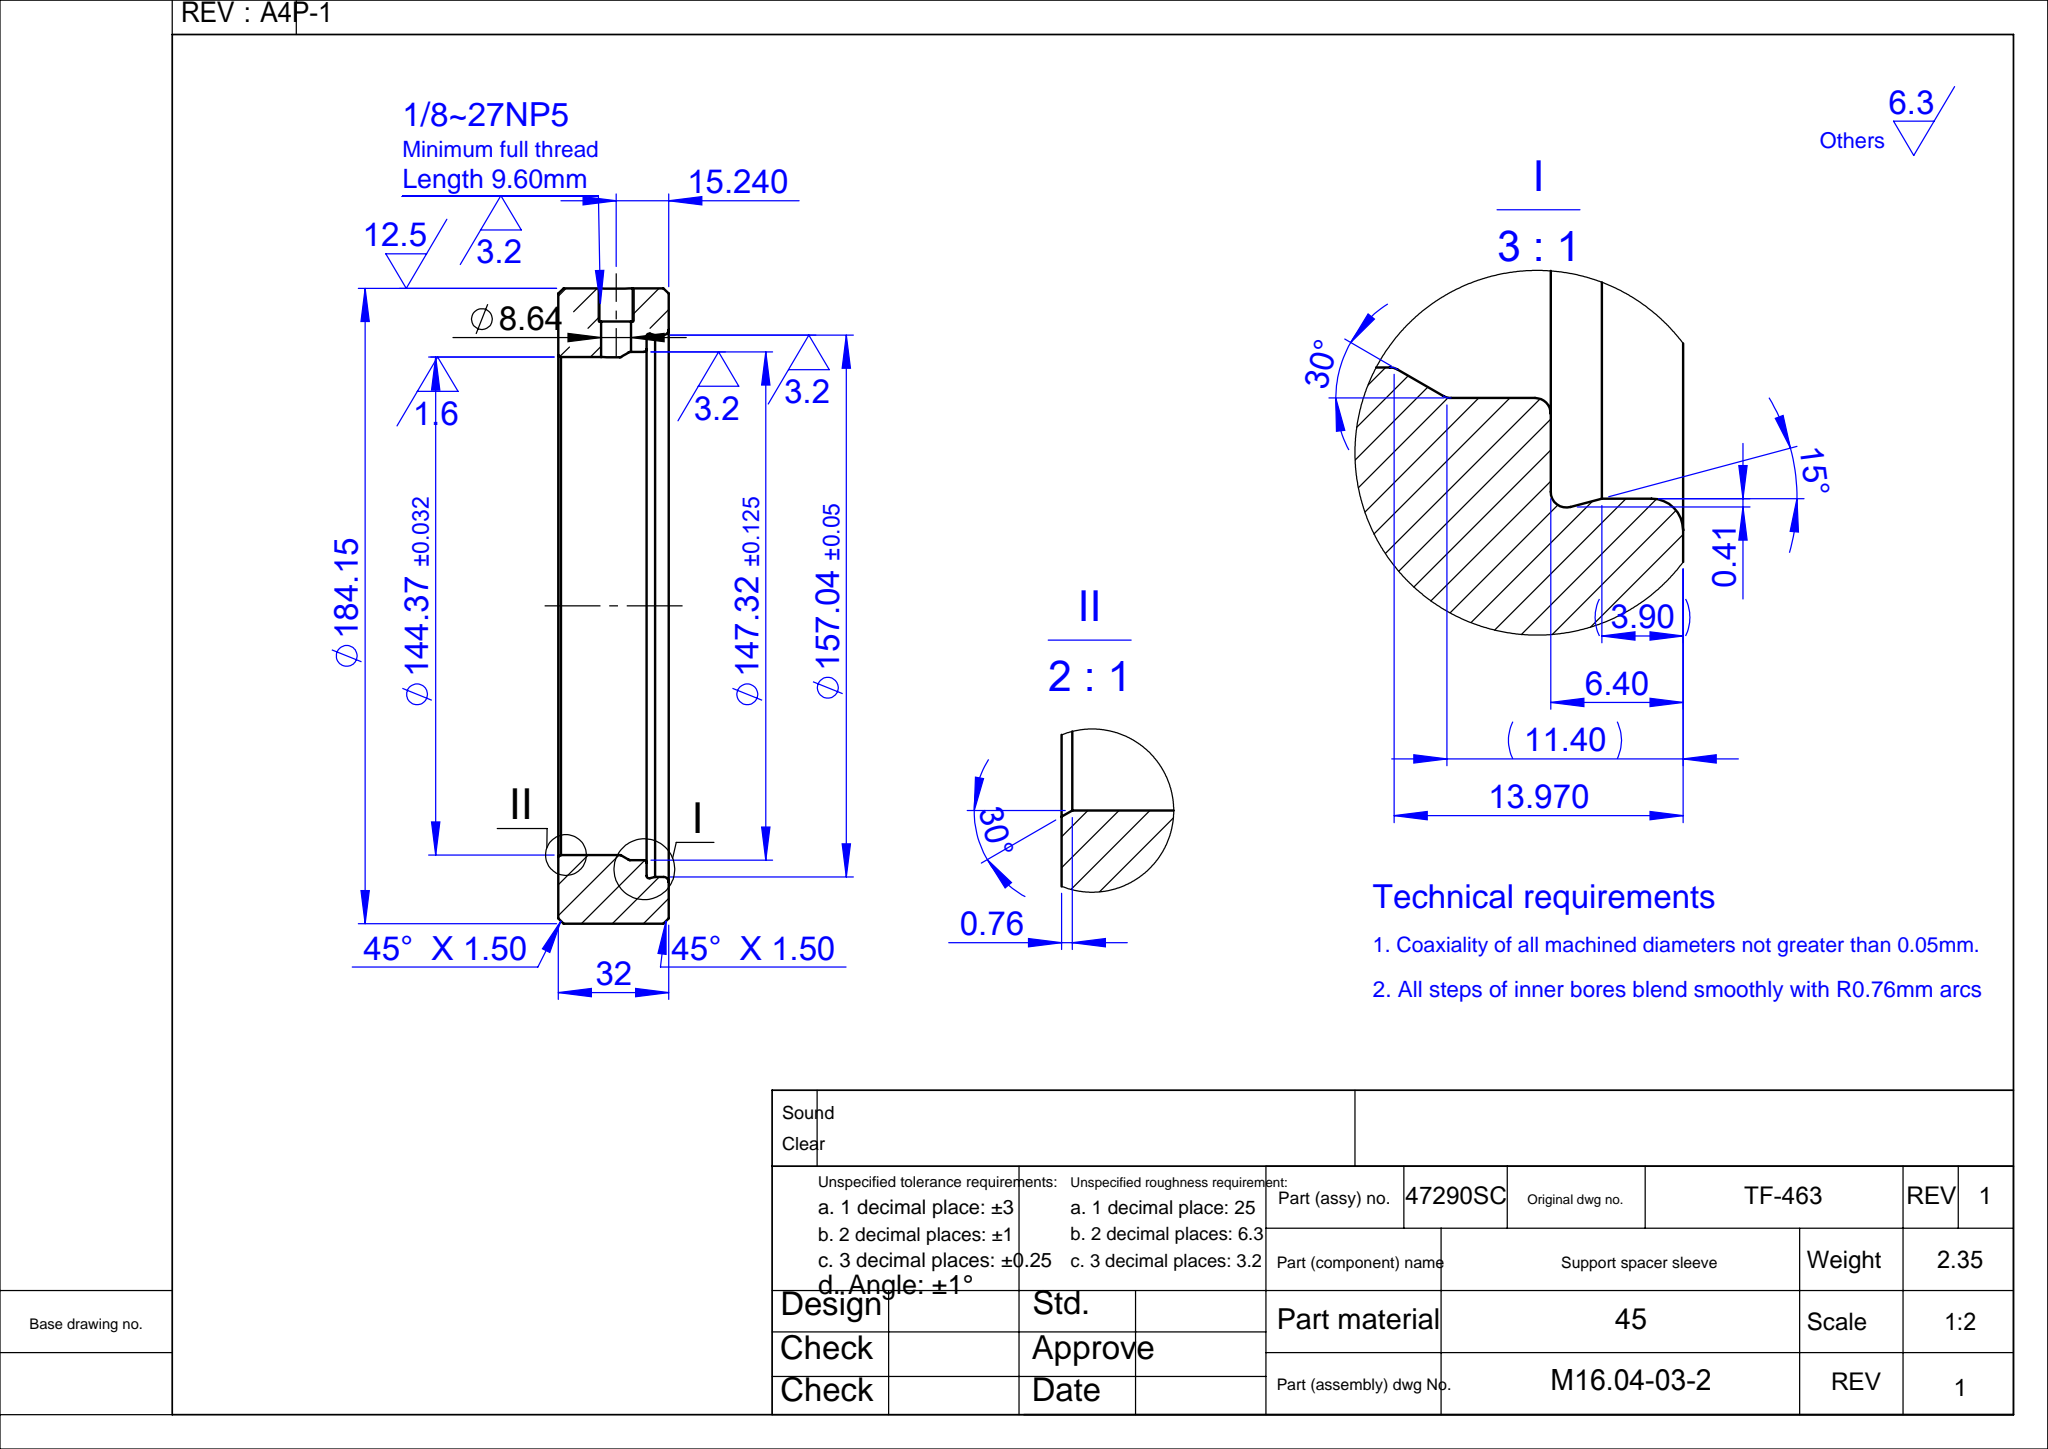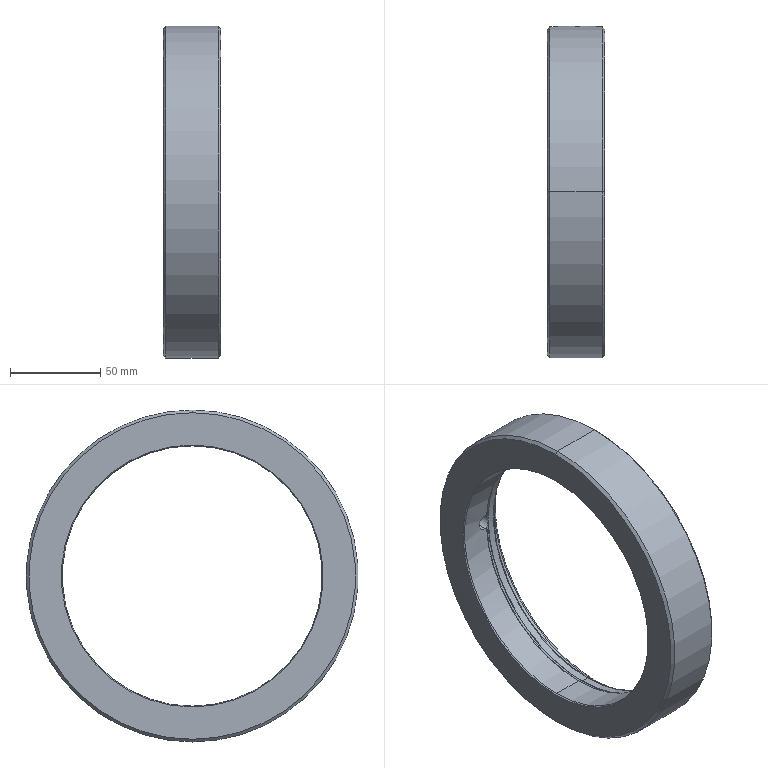Part | SolidWorks | features Chamfer 2, 3DProfileFeature 1, Cut 1, HoleWzd 1, Revolution 1 | 1 solid | 39 faces | box 32 x 184.15 x 184.15 mm | volume 301680 mm3 | cylinder 12 | torus 12 | cone 11 | plane 4 | commonest cylinder face diameters 8.636 x2 9.653 x2 144.374 x2 147.32 x2 157.04 x2 184.15 x2